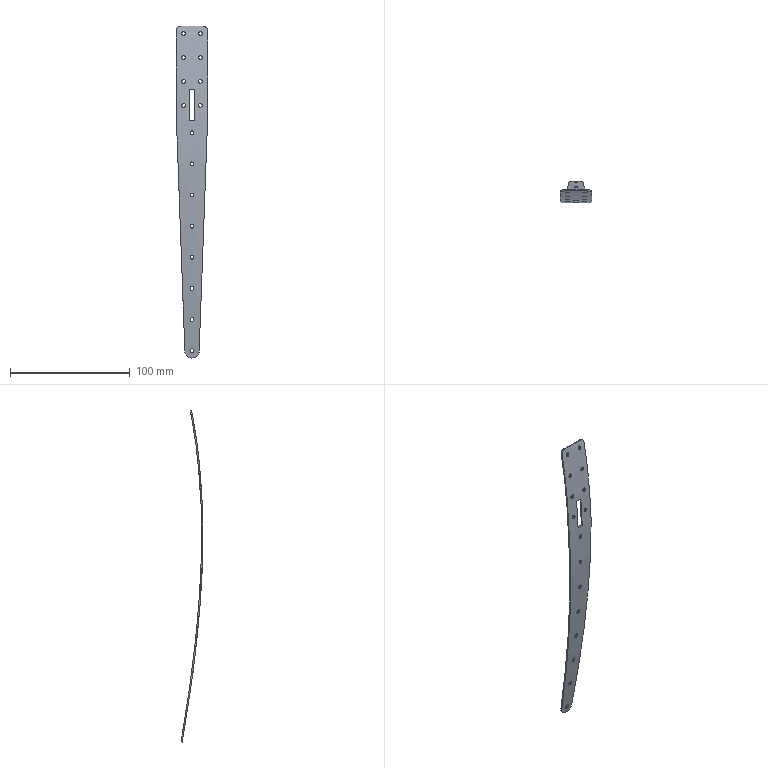Part | SolidWorks | features BaseBody 1 | 1 solid | 48 faces | box 26 x 18.209 x 277.366 mm | volume 5617 mm3 | cylinder 36 | plane 10 | spline 2 | commonest cylinder face diameters 3.2 x32 8 x2 12 x2